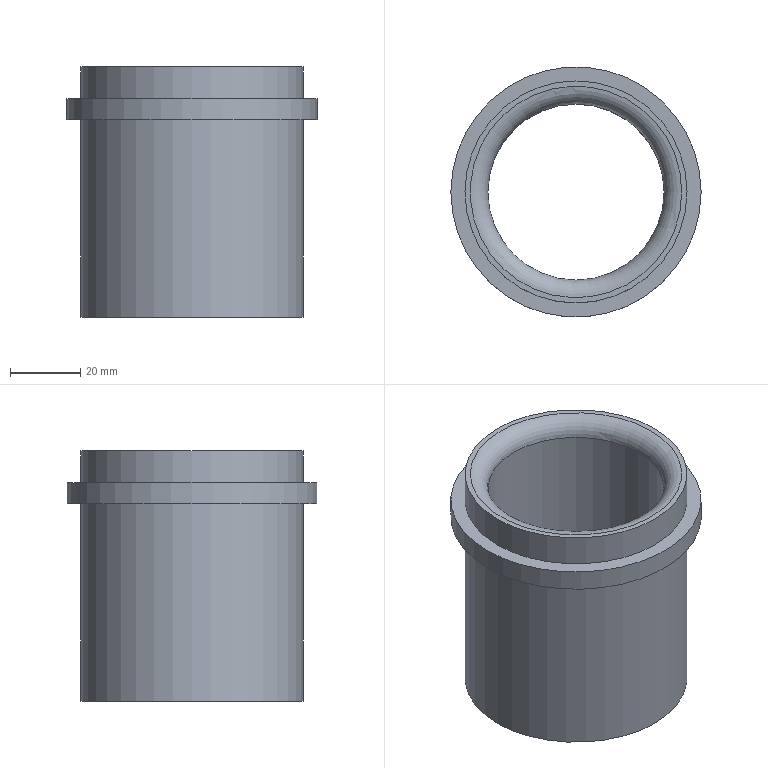Part | NX | features MAIN_BODY 2 | 1 solid | 10 faces | box 71 x 71 x 71 mm | volume 85950 mm3 | cylinder 4 | plane 4 | torus 2 | commonest cylinder face diameters 63 x2 50 x1 71 x1
STEP:
#1=CARTESIAN_POINT('',(1051.5,230.,179.));
#2=VERTEX_POINT('',#1);
#3=CARTESIAN_POINT('',(1020.,230.,179.));
#4=DIRECTION('',(0.,0.,-1.));
#5=DIRECTION('',(1.,0.,0.));
#6=AXIS2_PLACEMENT_3D('',#3,#4,#5);
#7=CIRCLE('',#6,31.5);
#8=EDGE_CURVE('',#2,#2,#7,.T.);
#9=ORIENTED_EDGE('',*,*,#8,.F.);
#10=EDGE_LOOP('',(#9));
#11=FACE_BOUND('',#10,.T.);
#12=CARTESIAN_POINT('',(1051.5,230.,235.));
#13=VERTEX_POINT('',#12);
#14=CARTESIAN_POINT('',(1020.,230.,235.));
#15=DIRECTION('',(0.,0.,-1.));
#16=DIRECTION('',(1.,0.,0.));
#17=AXIS2_PLACEMENT_3D('',#14,#15,#16);
#18=CIRCLE('',#17,31.5);
#19=EDGE_CURVE('',#13,#13,#18,.T.);
#20=ORIENTED_EDGE('',*,*,#19,.T.);
#21=EDGE_LOOP('',(#20));
#22=FACE_BOUND('',#21,.T.);
#23=CARTESIAN_POINT('',(1020.,230.,179.));
#24=DIRECTION('',(0.,0.,1.));
#25=DIRECTION('',(1.,0.,0.));
#26=AXIS2_PLACEMENT_3D('',#23,#24,#25);
#27=CYLINDRICAL_SURFACE('',#26,31.5);
#28=ADVANCED_FACE('',(#11,#22),#27,.T.);
#29=CARTESIAN_POINT('',(1045.,230.,181.));
#30=VERTEX_POINT('',#29);
#31=CARTESIAN_POINT('',(1020.,230.,181.));
#32=DIRECTION('',(0.,0.,-1.));
#33=DIRECTION('',(1.,0.,0.));
#34=AXIS2_PLACEMENT_3D('',#31,#32,#33);
#35=CIRCLE('',#34,25.);
#36=EDGE_CURVE('',#30,#30,#35,.F.);
#37=ORIENTED_EDGE('',*,*,#36,.F.);
#38=EDGE_LOOP('',(#37));
#39=FACE_BOUND('',#38,.T.);
#40=CARTESIAN_POINT('',(1045.,230.,245.));
#41=VERTEX_POINT('',#40);
#42=CARTESIAN_POINT('',(1020.,230.,245.));
#43=DIRECTION('',(0.,0.,-1.));
#44=DIRECTION('',(1.,0.,0.));
#45=AXIS2_PLACEMENT_3D('',#42,#43,#44);
#46=CIRCLE('',#45,25.);
#47=EDGE_CURVE('',#41,#41,#46,.T.);
#48=ORIENTED_EDGE('',*,*,#47,.F.);
#49=EDGE_LOOP('',(#48));
#50=FACE_BOUND('',#49,.T.);
#51=CARTESIAN_POINT('',(1020.,230.,179.));
#52=DIRECTION('',(0.,0.,1.));
#53=DIRECTION('',(1.,0.,0.));
#54=AXIS2_PLACEMENT_3D('',#51,#52,#53);
#55=CYLINDRICAL_SURFACE('',#54,25.);
#56=ADVANCED_FACE('',(#39,#50),#55,.F.);
#57=CARTESIAN_POINT('',(1051.5,230.,241.));
#58=VERTEX_POINT('',#57);
#59=CARTESIAN_POINT('',(1020.,230.,241.));
#60=DIRECTION('',(0.,0.,-1.));
#61=DIRECTION('',(1.,0.,0.));
#62=AXIS2_PLACEMENT_3D('',#59,#60,#61);
#63=CIRCLE('',#62,31.5);
#64=EDGE_CURVE('',#58,#58,#63,.F.);
#65=ORIENTED_EDGE('',*,*,#64,.T.);
#66=EDGE_LOOP('',(#65));
#67=FACE_BOUND('',#66,.T.);
#68=CARTESIAN_POINT('',(1051.5,230.,250.));
#69=VERTEX_POINT('',#68);
#70=CARTESIAN_POINT('',(1020.,230.,250.));
#71=DIRECTION('',(0.,0.,-1.));
#72=DIRECTION('',(1.,0.,0.));
#73=AXIS2_PLACEMENT_3D('',#70,#71,#72);
#74=CIRCLE('',#73,31.5);
#75=EDGE_CURVE('',#69,#69,#74,.T.);
#76=ORIENTED_EDGE('',*,*,#75,.T.);
#77=EDGE_LOOP('',(#76));
#78=FACE_BOUND('',#77,.T.);
#79=CARTESIAN_POINT('',(1020.,230.,179.));
#80=DIRECTION('',(0.,0.,1.));
#81=DIRECTION('',(1.,0.,0.));
#82=AXIS2_PLACEMENT_3D('',#79,#80,#81);
#83=CYLINDRICAL_SURFACE('',#82,31.5);
#84=ADVANCED_FACE('',(#67,#78),#83,.T.);
#85=CARTESIAN_POINT('',(1047.,230.,179.));
#86=VERTEX_POINT('',#85);
#87=CARTESIAN_POINT('',(1020.,230.,179.));
#88=DIRECTION('',(0.,0.,-1.));
#89=DIRECTION('',(1.,0.,0.));
#90=AXIS2_PLACEMENT_3D('',#87,#88,#89);
#91=CIRCLE('',#90,27.);
#92=EDGE_CURVE('',#86,#86,#91,.T.);
#93=ORIENTED_EDGE('',*,*,#92,.F.);
#94=EDGE_LOOP('',(#93));
#95=FACE_BOUND('',#94,.T.);
#96=ORIENTED_EDGE('',*,*,#8,.T.);
#97=EDGE_LOOP('',(#96));
#98=FACE_BOUND('',#97,.T.);
#99=CARTESIAN_POINT('',(1020.,230.,179.));
#100=DIRECTION('',(0.,0.,1.));
#101=DIRECTION('',(1.,0.,0.));
#102=AXIS2_PLACEMENT_3D('',#99,#100,#101);
#103=PLANE('',#102);
#104=ADVANCED_FACE('',(#95,#98),#103,.F.);
#105=CARTESIAN_POINT('',(1050.,230.,250.));
#106=VERTEX_POINT('',#105);
#107=CARTESIAN_POINT('',(1020.,230.,250.));
#108=DIRECTION('',(0.,0.,-1.));
#109=DIRECTION('',(1.,0.,0.));
#110=AXIS2_PLACEMENT_3D('',#107,#108,#109);
#111=CIRCLE('',#110,30.);
#112=EDGE_CURVE('',#106,#106,#111,.F.);
#113=ORIENTED_EDGE('',*,*,#112,.F.);
#114=EDGE_LOOP('',(#113));
#115=FACE_BOUND('',#114,.T.);
#116=ORIENTED_EDGE('',*,*,#75,.F.);
#117=EDGE_LOOP('',(#116));
#118=FACE_BOUND('',#117,.T.);
#119=CARTESIAN_POINT('',(1020.,230.,250.));
#120=DIRECTION('',(0.,0.,1.));
#121=DIRECTION('',(1.,0.,0.));
#122=AXIS2_PLACEMENT_3D('',#119,#120,#121);
#123=PLANE('',#122);
#124=ADVANCED_FACE('',(#115,#118),#123,.T.);
#125=CARTESIAN_POINT('',(1055.5,230.,241.));
#126=VERTEX_POINT('',#125);
#127=CARTESIAN_POINT('',(1020.,230.,241.));
#128=DIRECTION('',(0.,0.,-1.));
#129=DIRECTION('',(1.,0.,0.));
#130=AXIS2_PLACEMENT_3D('',#127,#128,#129);
#131=CIRCLE('',#130,35.5);
#132=EDGE_CURVE('',#126,#126,#131,.T.);
#133=ORIENTED_EDGE('',*,*,#132,.T.);
#134=EDGE_LOOP('',(#133));
#135=FACE_BOUND('',#134,.T.);
#136=CARTESIAN_POINT('',(1055.5,230.,235.));
#137=VERTEX_POINT('',#136);
#138=CARTESIAN_POINT('',(1020.,230.,235.));
#139=DIRECTION('',(0.,0.,-1.));
#140=DIRECTION('',(1.,0.,0.));
#141=AXIS2_PLACEMENT_3D('',#138,#139,#140);
#142=CIRCLE('',#141,35.5);
#143=EDGE_CURVE('',#137,#137,#142,.T.);
#144=ORIENTED_EDGE('',*,*,#143,.F.);
#145=EDGE_LOOP('',(#144));
#146=FACE_BOUND('',#145,.T.);
#147=CARTESIAN_POINT('',(1020.,230.,241.));
#148=DIRECTION('',(0.,0.,-1.));
#149=DIRECTION('',(-1.,0.,0.));
#150=AXIS2_PLACEMENT_3D('',#147,#148,#149);
#151=CYLINDRICAL_SURFACE('',#150,35.5);
#152=ADVANCED_FACE('',(#135,#146),#151,.T.);
#153=ORIENTED_EDGE('',*,*,#64,.F.);
#154=EDGE_LOOP('',(#153));
#155=FACE_BOUND('',#154,.T.);
#156=ORIENTED_EDGE('',*,*,#132,.F.);
#157=EDGE_LOOP('',(#156));
#158=FACE_BOUND('',#157,.T.);
#159=CARTESIAN_POINT('',(1020.,230.,241.));
#160=DIRECTION('',(0.,0.,1.));
#161=DIRECTION('',(1.,0.,0.));
#162=AXIS2_PLACEMENT_3D('',#159,#160,#161);
#163=PLANE('',#162);
#164=ADVANCED_FACE('',(#155,#158),#163,.T.);
#165=ORIENTED_EDGE('',*,*,#19,.F.);
#166=EDGE_LOOP('',(#165));
#167=FACE_BOUND('',#166,.T.);
#168=ORIENTED_EDGE('',*,*,#143,.T.);
#169=EDGE_LOOP('',(#168));
#170=FACE_BOUND('',#169,.T.);
#171=CARTESIAN_POINT('',(1020.,230.,235.));
#172=DIRECTION('',(0.,0.,1.));
#173=DIRECTION('',(1.,0.,0.));
#174=AXIS2_PLACEMENT_3D('',#171,#172,#173);
#175=PLANE('',#174);
#176=ADVANCED_FACE('',(#167,#170),#175,.F.);
#177=ORIENTED_EDGE('',*,*,#112,.T.);
#178=EDGE_LOOP('',(#177));
#179=FACE_BOUND('',#178,.T.);
#180=ORIENTED_EDGE('',*,*,#47,.T.);
#181=EDGE_LOOP('',(#180));
#182=FACE_BOUND('',#181,.T.);
#183=CARTESIAN_POINT('',(1020.,230.,245.));
#184=DIRECTION('',(0.,0.,1.));
#185=DIRECTION('',(1.,0.,0.));
#186=AXIS2_PLACEMENT_3D('',#183,#184,#185);
#187=TOROIDAL_SURFACE('',#186,30.,5.);
#188=ADVANCED_FACE('',(#179,#182),#187,.T.);
#189=ORIENTED_EDGE('',*,*,#36,.T.);
#190=EDGE_LOOP('',(#189));
#191=FACE_BOUND('',#190,.T.);
#192=ORIENTED_EDGE('',*,*,#92,.T.);
#193=EDGE_LOOP('',(#192));
#194=FACE_BOUND('',#193,.T.);
#195=CARTESIAN_POINT('',(1020.,230.,181.));
#196=DIRECTION('',(0.,0.,1.));
#197=DIRECTION('',(1.,0.,0.));
#198=AXIS2_PLACEMENT_3D('',#195,#196,#197);
#199=TOROIDAL_SURFACE('',#198,27.,2.);
#200=ADVANCED_FACE('',(#191,#194),#199,.T.);
#201=CLOSED_SHELL('',(#28,#56,#84,#104,#124,#152,#164,#176,#188,#200));
#202=MANIFOLD_SOLID_BREP('',#201);
#203=(LENGTH_UNIT()NAMED_UNIT(*)SI_UNIT(.MILLI.,.METRE.));
#204=UNCERTAINTY_MEASURE_WITH_UNIT(LENGTH_MEASURE(0.00001),#203,'','');
#205=(NAMED_UNIT(*)PLANE_ANGLE_UNIT()SI_UNIT($,.RADIAN.));
#206=(NAMED_UNIT(*)SI_UNIT($,.STERADIAN.)SOLID_ANGLE_UNIT());
#207=(GEOMETRIC_REPRESENTATION_CONTEXT(3)GLOBAL_UNCERTAINTY_ASSIGNED_CONTEXT((#204))GLOBAL_UNIT_ASSIGNED_CONTEXT((#203,#205,#206))REPRESENTATION_CONTEXT('',''));
#208=ADVANCED_BREP_SHAPE_REPRESENTATION('',(#202),#207);